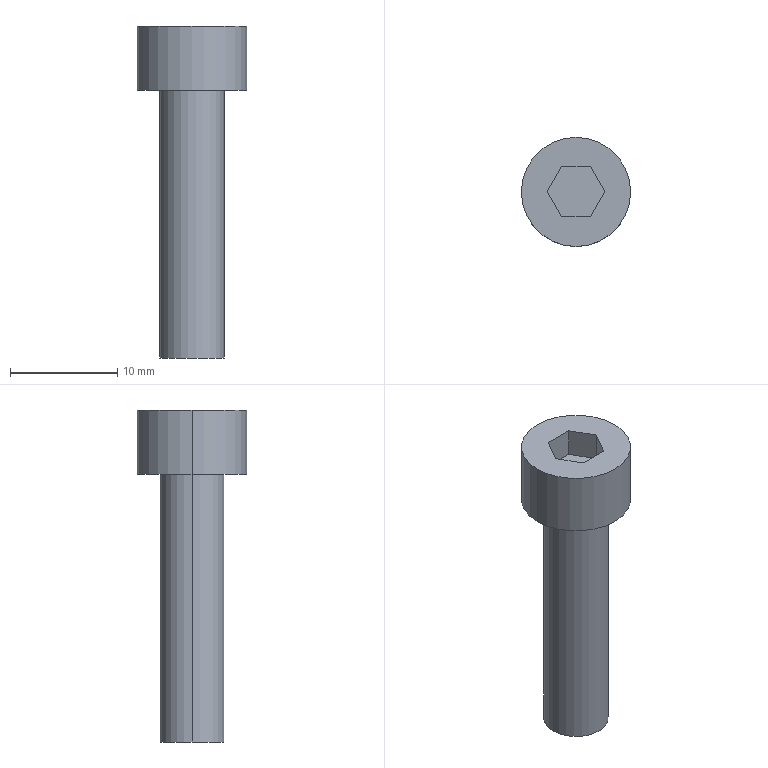Part | SolidWorks | features BaseBody 1 | 1 solid | 14 faces | box 10.2 x 10.2 x 31 mm | volume 1146 mm3 | plane 10 | cylinder 4 | commonest cylinder face diameters 6 x2 10.2 x2
STEP:
#1=CARTESIAN_POINT('',(3.,0.,-25.));
#2=VERTEX_POINT('',#1);
#3=CARTESIAN_POINT('',(-3.,0.,-25.));
#4=VERTEX_POINT('',#3);
#5=CARTESIAN_POINT('',(0.,0.,-25.));
#6=DIRECTION('',(0.,0.,1.));
#7=DIRECTION('',(1.,0.,0.));
#8=AXIS2_PLACEMENT_3D('',#5,#6,#7);
#9=CIRCLE('',#8,3.);
#10=EDGE_CURVE('',#2,#4,#9,.T.);
#11=ORIENTED_EDGE('',*,*,#10,.T.);
#12=CARTESIAN_POINT('',(-3.,0.,0.));
#13=VERTEX_POINT('',#12);
#14=CARTESIAN_POINT('',(-3.,0.,-25.));
#15=DIRECTION('',(0.,0.,1.));
#16=VECTOR('',#15,1000.);
#17=LINE('',#14,#16);
#18=EDGE_CURVE('',#4,#13,#17,.T.);
#19=ORIENTED_EDGE('',*,*,#18,.T.);
#20=CARTESIAN_POINT('',(3.,0.,0.));
#21=VERTEX_POINT('',#20);
#22=CARTESIAN_POINT('',(0.,0.,0.));
#23=DIRECTION('',(0.,0.,-1.));
#24=DIRECTION('',(1.,0.,0.));
#25=AXIS2_PLACEMENT_3D('',#22,#23,#24);
#26=CIRCLE('',#25,3.);
#27=EDGE_CURVE('',#13,#21,#26,.T.);
#28=ORIENTED_EDGE('',*,*,#27,.T.);
#29=CARTESIAN_POINT('',(3.,0.,-25.));
#30=DIRECTION('',(0.,0.,1.));
#31=VECTOR('',#30,1000.);
#32=LINE('',#29,#31);
#33=EDGE_CURVE('',#2,#21,#32,.T.);
#34=ORIENTED_EDGE('',*,*,#33,.F.);
#35=EDGE_LOOP('',(#11,#19,#28,#34));
#36=FACE_OUTER_BOUND('',#35,.T.);
#37=CARTESIAN_POINT('',(0.,0.,-25.));
#38=DIRECTION('',(0.,0.,1.));
#39=DIRECTION('',(1.,0.,0.));
#40=AXIS2_PLACEMENT_3D('',#37,#38,#39);
#41=CYLINDRICAL_SURFACE('',#40,3.);
#42=ADVANCED_FACE('',(#36),#41,.T.);
#43=CARTESIAN_POINT('',(5.1,0.,0.));
#44=VERTEX_POINT('',#43);
#45=CARTESIAN_POINT('',(-5.1,0.,0.));
#46=VERTEX_POINT('',#45);
#47=CARTESIAN_POINT('',(0.,0.,0.));
#48=DIRECTION('',(0.,0.,1.));
#49=DIRECTION('',(1.,0.,0.));
#50=AXIS2_PLACEMENT_3D('',#47,#48,#49);
#51=CIRCLE('',#50,5.1);
#52=EDGE_CURVE('',#44,#46,#51,.T.);
#53=ORIENTED_EDGE('',*,*,#52,.T.);
#54=CARTESIAN_POINT('',(-5.1,0.,6.));
#55=VERTEX_POINT('',#54);
#56=CARTESIAN_POINT('',(-5.1,0.,0.));
#57=DIRECTION('',(0.,0.,1.));
#58=VECTOR('',#57,1000.);
#59=LINE('',#56,#58);
#60=EDGE_CURVE('',#46,#55,#59,.T.);
#61=ORIENTED_EDGE('',*,*,#60,.T.);
#62=CARTESIAN_POINT('',(5.1,0.,6.));
#63=VERTEX_POINT('',#62);
#64=CARTESIAN_POINT('',(0.,0.,6.));
#65=DIRECTION('',(0.,0.,-1.));
#66=DIRECTION('',(1.,0.,0.));
#67=AXIS2_PLACEMENT_3D('',#64,#65,#66);
#68=CIRCLE('',#67,5.1);
#69=EDGE_CURVE('',#55,#63,#68,.T.);
#70=ORIENTED_EDGE('',*,*,#69,.T.);
#71=CARTESIAN_POINT('',(5.1,0.,0.));
#72=DIRECTION('',(0.,0.,1.));
#73=VECTOR('',#72,1000.);
#74=LINE('',#71,#73);
#75=EDGE_CURVE('',#44,#63,#74,.T.);
#76=ORIENTED_EDGE('',*,*,#75,.F.);
#77=EDGE_LOOP('',(#53,#61,#70,#76));
#78=FACE_OUTER_BOUND('',#77,.T.);
#79=CARTESIAN_POINT('',(0.,0.,0.));
#80=DIRECTION('',(0.,0.,1.));
#81=DIRECTION('',(1.,0.,0.));
#82=AXIS2_PLACEMENT_3D('',#79,#80,#81);
#83=CYLINDRICAL_SURFACE('',#82,5.1);
#84=ADVANCED_FACE('',(#78),#83,.T.);
#85=ORIENTED_EDGE('',*,*,#18,.F.);
#86=CARTESIAN_POINT('',(0.,0.,-25.));
#87=DIRECTION('',(0.,0.,1.));
#88=DIRECTION('',(1.,0.,0.));
#89=AXIS2_PLACEMENT_3D('',#86,#87,#88);
#90=CIRCLE('',#89,3.);
#91=EDGE_CURVE('',#4,#2,#90,.T.);
#92=ORIENTED_EDGE('',*,*,#91,.T.);
#93=ORIENTED_EDGE('',*,*,#33,.T.);
#94=CARTESIAN_POINT('',(0.,0.,0.));
#95=DIRECTION('',(0.,0.,-1.));
#96=DIRECTION('',(1.,0.,0.));
#97=AXIS2_PLACEMENT_3D('',#94,#95,#96);
#98=CIRCLE('',#97,3.);
#99=EDGE_CURVE('',#21,#13,#98,.T.);
#100=ORIENTED_EDGE('',*,*,#99,.T.);
#101=EDGE_LOOP('',(#85,#92,#93,#100));
#102=FACE_OUTER_BOUND('',#101,.T.);
#103=CARTESIAN_POINT('',(0.,0.,-25.));
#104=DIRECTION('',(0.,0.,1.));
#105=DIRECTION('',(1.,0.,0.));
#106=AXIS2_PLACEMENT_3D('',#103,#104,#105);
#107=CYLINDRICAL_SURFACE('',#106,3.);
#108=ADVANCED_FACE('',(#102),#107,.T.);
#109=ORIENTED_EDGE('',*,*,#10,.F.);
#110=ORIENTED_EDGE('',*,*,#91,.F.);
#111=EDGE_LOOP('',(#109,#110));
#112=FACE_OUTER_BOUND('',#111,.T.);
#113=CARTESIAN_POINT('',(0.,0.,-25.));
#114=DIRECTION('',(0.,0.,1.));
#115=DIRECTION('',(1.,0.,0.));
#116=AXIS2_PLACEMENT_3D('',#113,#114,#115);
#117=PLANE('',#116);
#118=ADVANCED_FACE('',(#112),#117,.F.);
#119=ORIENTED_EDGE('',*,*,#99,.F.);
#120=ORIENTED_EDGE('',*,*,#27,.F.);
#121=EDGE_LOOP('',(#119,#120));
#122=FACE_BOUND('',#121,.T.);
#123=ORIENTED_EDGE('',*,*,#52,.F.);
#124=CARTESIAN_POINT('',(0.,0.,0.));
#125=DIRECTION('',(0.,0.,1.));
#126=DIRECTION('',(1.,0.,0.));
#127=AXIS2_PLACEMENT_3D('',#124,#125,#126);
#128=CIRCLE('',#127,5.1);
#129=EDGE_CURVE('',#46,#44,#128,.T.);
#130=ORIENTED_EDGE('',*,*,#129,.F.);
#131=EDGE_LOOP('',(#123,#130));
#132=FACE_OUTER_BOUND('',#131,.T.);
#133=CARTESIAN_POINT('',(0.,0.,0.));
#134=DIRECTION('',(0.,0.,1.));
#135=DIRECTION('',(1.,0.,0.));
#136=AXIS2_PLACEMENT_3D('',#133,#134,#135);
#137=PLANE('',#136);
#138=ADVANCED_FACE('',(#122,#132),#137,.F.);
#139=ORIENTED_EDGE('',*,*,#60,.F.);
#140=ORIENTED_EDGE('',*,*,#129,.T.);
#141=ORIENTED_EDGE('',*,*,#75,.T.);
#142=CARTESIAN_POINT('',(0.,0.,6.));
#143=DIRECTION('',(0.,0.,-1.));
#144=DIRECTION('',(1.,0.,0.));
#145=AXIS2_PLACEMENT_3D('',#142,#143,#144);
#146=CIRCLE('',#145,5.1);
#147=EDGE_CURVE('',#63,#55,#146,.T.);
#148=ORIENTED_EDGE('',*,*,#147,.T.);
#149=EDGE_LOOP('',(#139,#140,#141,#148));
#150=FACE_OUTER_BOUND('',#149,.T.);
#151=CARTESIAN_POINT('',(0.,0.,0.));
#152=DIRECTION('',(0.,0.,1.));
#153=DIRECTION('',(1.,0.,0.));
#154=AXIS2_PLACEMENT_3D('',#151,#152,#153);
#155=CYLINDRICAL_SURFACE('',#154,5.1);
#156=ADVANCED_FACE('',(#150),#155,.T.);
#157=CARTESIAN_POINT('',(-1.35,-2.338,6.));
#158=VERTEX_POINT('',#157);
#159=CARTESIAN_POINT('',(-2.7,0.,6.));
#160=VERTEX_POINT('',#159);
#161=CARTESIAN_POINT('',(-1.35,-2.338,6.));
#162=DIRECTION('',(-0.5,0.866,0.));
#163=VECTOR('',#162,1000.);
#164=LINE('',#161,#163);
#165=EDGE_CURVE('',#158,#160,#164,.T.);
#166=ORIENTED_EDGE('',*,*,#165,.T.);
#167=CARTESIAN_POINT('',(-1.35,2.338,6.));
#168=VERTEX_POINT('',#167);
#169=CARTESIAN_POINT('',(-2.7,0.,6.));
#170=DIRECTION('',(0.5,0.866,0.));
#171=VECTOR('',#170,1000.);
#172=LINE('',#169,#171);
#173=EDGE_CURVE('',#160,#168,#172,.T.);
#174=ORIENTED_EDGE('',*,*,#173,.T.);
#175=CARTESIAN_POINT('',(1.35,2.338,6.));
#176=VERTEX_POINT('',#175);
#177=CARTESIAN_POINT('',(0.,2.338,6.));
#178=DIRECTION('',(1.,0.,0.));
#179=VECTOR('',#178,1000.);
#180=LINE('',#177,#179);
#181=EDGE_CURVE('',#168,#176,#180,.T.);
#182=ORIENTED_EDGE('',*,*,#181,.T.);
#183=CARTESIAN_POINT('',(2.7,0.,6.));
#184=VERTEX_POINT('',#183);
#185=CARTESIAN_POINT('',(1.35,2.338,6.));
#186=DIRECTION('',(0.5,-0.866,0.));
#187=VECTOR('',#186,1000.);
#188=LINE('',#185,#187);
#189=EDGE_CURVE('',#176,#184,#188,.T.);
#190=ORIENTED_EDGE('',*,*,#189,.T.);
#191=CARTESIAN_POINT('',(1.35,-2.338,6.));
#192=VERTEX_POINT('',#191);
#193=CARTESIAN_POINT('',(2.7,0.,6.));
#194=DIRECTION('',(-0.5,-0.866,0.));
#195=VECTOR('',#194,1000.);
#196=LINE('',#193,#195);
#197=EDGE_CURVE('',#184,#192,#196,.T.);
#198=ORIENTED_EDGE('',*,*,#197,.T.);
#199=CARTESIAN_POINT('',(0.,-2.338,6.));
#200=DIRECTION('',(-1.,0.,0.));
#201=VECTOR('',#200,1000.);
#202=LINE('',#199,#201);
#203=EDGE_CURVE('',#192,#158,#202,.T.);
#204=ORIENTED_EDGE('',*,*,#203,.T.);
#205=EDGE_LOOP('',(#166,#174,#182,#190,#198,#204));
#206=FACE_BOUND('',#205,.T.);
#207=ORIENTED_EDGE('',*,*,#147,.F.);
#208=ORIENTED_EDGE('',*,*,#69,.F.);
#209=EDGE_LOOP('',(#207,#208));
#210=FACE_OUTER_BOUND('',#209,.T.);
#211=CARTESIAN_POINT('',(0.,0.,6.));
#212=DIRECTION('',(0.,0.,1.));
#213=DIRECTION('',(1.,0.,0.));
#214=AXIS2_PLACEMENT_3D('',#211,#212,#213);
#215=PLANE('',#214);
#216=ADVANCED_FACE('',(#206,#210),#215,.T.);
#217=ORIENTED_EDGE('',*,*,#173,.F.);
#218=CARTESIAN_POINT('',(-2.7,0.,3.3));
#219=VERTEX_POINT('',#218);
#220=CARTESIAN_POINT('',(-2.7,0.,3.3));
#221=DIRECTION('',(0.,0.,-1.));
#222=VECTOR('',#221,1000.);
#223=LINE('',#220,#222);
#224=EDGE_CURVE('',#160,#219,#223,.T.);
#225=ORIENTED_EDGE('',*,*,#224,.T.);
#226=CARTESIAN_POINT('',(-1.35,2.338,3.3));
#227=VERTEX_POINT('',#226);
#228=CARTESIAN_POINT('',(-1.35,2.338,3.3));
#229=DIRECTION('',(0.5,0.866,0.));
#230=VECTOR('',#229,1000.);
#231=LINE('',#228,#230);
#232=EDGE_CURVE('',#219,#227,#231,.T.);
#233=ORIENTED_EDGE('',*,*,#232,.T.);
#234=CARTESIAN_POINT('',(-1.35,2.338,3.3));
#235=DIRECTION('',(0.,0.,1.));
#236=VECTOR('',#235,1000.);
#237=LINE('',#234,#236);
#238=EDGE_CURVE('',#227,#168,#237,.T.);
#239=ORIENTED_EDGE('',*,*,#238,.T.);
#240=EDGE_LOOP('',(#217,#225,#233,#239));
#241=FACE_OUTER_BOUND('',#240,.T.);
#242=CARTESIAN_POINT('',(-1.35,2.338,3.3));
#243=DIRECTION('',(0.866,-0.5,0.));
#244=DIRECTION('',(0.5,0.866,0.));
#245=AXIS2_PLACEMENT_3D('',#242,#243,#244);
#246=PLANE('',#245);
#247=ADVANCED_FACE('',(#241),#246,.T.);
#248=ORIENTED_EDGE('',*,*,#165,.F.);
#249=CARTESIAN_POINT('',(-1.35,-2.338,3.3));
#250=VERTEX_POINT('',#249);
#251=CARTESIAN_POINT('',(-1.35,-2.338,3.3));
#252=DIRECTION('',(0.,0.,-1.));
#253=VECTOR('',#252,1000.);
#254=LINE('',#251,#253);
#255=EDGE_CURVE('',#158,#250,#254,.T.);
#256=ORIENTED_EDGE('',*,*,#255,.T.);
#257=CARTESIAN_POINT('',(-2.7,0.,3.3));
#258=DIRECTION('',(-0.5,0.866,0.));
#259=VECTOR('',#258,1000.);
#260=LINE('',#257,#259);
#261=EDGE_CURVE('',#250,#219,#260,.T.);
#262=ORIENTED_EDGE('',*,*,#261,.T.);
#263=ORIENTED_EDGE('',*,*,#224,.F.);
#264=EDGE_LOOP('',(#248,#256,#262,#263));
#265=FACE_OUTER_BOUND('',#264,.T.);
#266=CARTESIAN_POINT('',(-2.7,0.,3.3));
#267=DIRECTION('',(0.866,0.5,0.));
#268=DIRECTION('',(-0.5,0.866,0.));
#269=AXIS2_PLACEMENT_3D('',#266,#267,#268);
#270=PLANE('',#269);
#271=ADVANCED_FACE('',(#265),#270,.T.);
#272=ORIENTED_EDGE('',*,*,#203,.F.);
#273=CARTESIAN_POINT('',(1.35,-2.338,3.3));
#274=VERTEX_POINT('',#273);
#275=CARTESIAN_POINT('',(1.35,-2.338,3.3));
#276=DIRECTION('',(0.,0.,-1.));
#277=VECTOR('',#276,1000.);
#278=LINE('',#275,#277);
#279=EDGE_CURVE('',#192,#274,#278,.T.);
#280=ORIENTED_EDGE('',*,*,#279,.T.);
#281=CARTESIAN_POINT('',(-1.35,-2.338,3.3));
#282=DIRECTION('',(-1.,0.,0.));
#283=VECTOR('',#282,1000.);
#284=LINE('',#281,#283);
#285=EDGE_CURVE('',#274,#250,#284,.T.);
#286=ORIENTED_EDGE('',*,*,#285,.T.);
#287=ORIENTED_EDGE('',*,*,#255,.F.);
#288=EDGE_LOOP('',(#272,#280,#286,#287));
#289=FACE_OUTER_BOUND('',#288,.T.);
#290=CARTESIAN_POINT('',(-1.35,-2.338,3.3));
#291=DIRECTION('',(0.,1.,0.));
#292=DIRECTION('',(-1.,0.,0.));
#293=AXIS2_PLACEMENT_3D('',#290,#291,#292);
#294=PLANE('',#293);
#295=ADVANCED_FACE('',(#289),#294,.T.);
#296=ORIENTED_EDGE('',*,*,#197,.F.);
#297=CARTESIAN_POINT('',(2.7,0.,3.3));
#298=VERTEX_POINT('',#297);
#299=CARTESIAN_POINT('',(2.7,0.,3.3));
#300=DIRECTION('',(0.,0.,-1.));
#301=VECTOR('',#300,1000.);
#302=LINE('',#299,#301);
#303=EDGE_CURVE('',#184,#298,#302,.T.);
#304=ORIENTED_EDGE('',*,*,#303,.T.);
#305=CARTESIAN_POINT('',(1.35,-2.338,3.3));
#306=DIRECTION('',(-0.5,-0.866,0.));
#307=VECTOR('',#306,1000.);
#308=LINE('',#305,#307);
#309=EDGE_CURVE('',#298,#274,#308,.T.);
#310=ORIENTED_EDGE('',*,*,#309,.T.);
#311=ORIENTED_EDGE('',*,*,#279,.F.);
#312=EDGE_LOOP('',(#296,#304,#310,#311));
#313=FACE_OUTER_BOUND('',#312,.T.);
#314=CARTESIAN_POINT('',(1.35,-2.338,3.3));
#315=DIRECTION('',(-0.866,0.5,0.));
#316=DIRECTION('',(-0.5,-0.866,0.));
#317=AXIS2_PLACEMENT_3D('',#314,#315,#316);
#318=PLANE('',#317);
#319=ADVANCED_FACE('',(#313),#318,.T.);
#320=ORIENTED_EDGE('',*,*,#189,.F.);
#321=CARTESIAN_POINT('',(1.35,2.338,3.3));
#322=VERTEX_POINT('',#321);
#323=CARTESIAN_POINT('',(1.35,2.338,3.3));
#324=DIRECTION('',(0.,0.,-1.));
#325=VECTOR('',#324,1000.);
#326=LINE('',#323,#325);
#327=EDGE_CURVE('',#176,#322,#326,.T.);
#328=ORIENTED_EDGE('',*,*,#327,.T.);
#329=CARTESIAN_POINT('',(2.7,0.,3.3));
#330=DIRECTION('',(0.5,-0.866,0.));
#331=VECTOR('',#330,1000.);
#332=LINE('',#329,#331);
#333=EDGE_CURVE('',#322,#298,#332,.T.);
#334=ORIENTED_EDGE('',*,*,#333,.T.);
#335=ORIENTED_EDGE('',*,*,#303,.F.);
#336=EDGE_LOOP('',(#320,#328,#334,#335));
#337=FACE_OUTER_BOUND('',#336,.T.);
#338=CARTESIAN_POINT('',(2.7,0.,3.3));
#339=DIRECTION('',(-0.866,-0.5,0.));
#340=DIRECTION('',(0.5,-0.866,0.));
#341=AXIS2_PLACEMENT_3D('',#338,#339,#340);
#342=PLANE('',#341);
#343=ADVANCED_FACE('',(#337),#342,.T.);
#344=ORIENTED_EDGE('',*,*,#181,.F.);
#345=ORIENTED_EDGE('',*,*,#238,.F.);
#346=CARTESIAN_POINT('',(1.35,2.338,3.3));
#347=DIRECTION('',(1.,0.,0.));
#348=VECTOR('',#347,1000.);
#349=LINE('',#346,#348);
#350=EDGE_CURVE('',#227,#322,#349,.T.);
#351=ORIENTED_EDGE('',*,*,#350,.T.);
#352=ORIENTED_EDGE('',*,*,#327,.F.);
#353=EDGE_LOOP('',(#344,#345,#351,#352));
#354=FACE_OUTER_BOUND('',#353,.T.);
#355=CARTESIAN_POINT('',(1.35,2.338,3.3));
#356=DIRECTION('',(0.,-1.,0.));
#357=DIRECTION('',(0.,0.,-1.));
#358=AXIS2_PLACEMENT_3D('',#355,#356,#357);
#359=PLANE('',#358);
#360=ADVANCED_FACE('',(#354),#359,.T.);
#361=ORIENTED_EDGE('',*,*,#285,.F.);
#362=ORIENTED_EDGE('',*,*,#309,.F.);
#363=ORIENTED_EDGE('',*,*,#333,.F.);
#364=ORIENTED_EDGE('',*,*,#350,.F.);
#365=ORIENTED_EDGE('',*,*,#232,.F.);
#366=ORIENTED_EDGE('',*,*,#261,.F.);
#367=EDGE_LOOP('',(#361,#362,#363,#364,#365,#366));
#368=FACE_OUTER_BOUND('',#367,.T.);
#369=CARTESIAN_POINT('',(0.,0.,3.3));
#370=DIRECTION('',(0.,0.,1.));
#371=DIRECTION('',(1.,0.,0.));
#372=AXIS2_PLACEMENT_3D('',#369,#370,#371);
#373=PLANE('',#372);
#374=ADVANCED_FACE('',(#368),#373,.T.);
#375=CLOSED_SHELL('',(#42,#84,#108,#118,#138,#156,#216,#247,#271,#295,#319,#343,#360,#374));
#376=MANIFOLD_SOLID_BREP('',#375);
#377=CARTESIAN_POINT('',(0.,0.,0.));
#378=DIRECTION('',(0.,0.,1.));
#379=DIRECTION('',(1.,0.,0.));
#380=AXIS2_PLACEMENT_3D('',#377,#378,#379);
#381=(LENGTH_UNIT()NAMED_UNIT(*)SI_UNIT(.MILLI.,.METRE.));
#382=UNCERTAINTY_MEASURE_WITH_UNIT(LENGTH_MEASURE(0.00001),#381,'','');
#383=(NAMED_UNIT(*)PLANE_ANGLE_UNIT()SI_UNIT($,.RADIAN.));
#384=(NAMED_UNIT(*)SI_UNIT($,.STERADIAN.)SOLID_ANGLE_UNIT());
#385=(GEOMETRIC_REPRESENTATION_CONTEXT(3)GLOBAL_UNCERTAINTY_ASSIGNED_CONTEXT((#382))GLOBAL_UNIT_ASSIGNED_CONTEXT((#381,#383,#384))REPRESENTATION_CONTEXT('',''));
#386=ADVANCED_BREP_SHAPE_REPRESENTATION('',(#376,#380),#385);